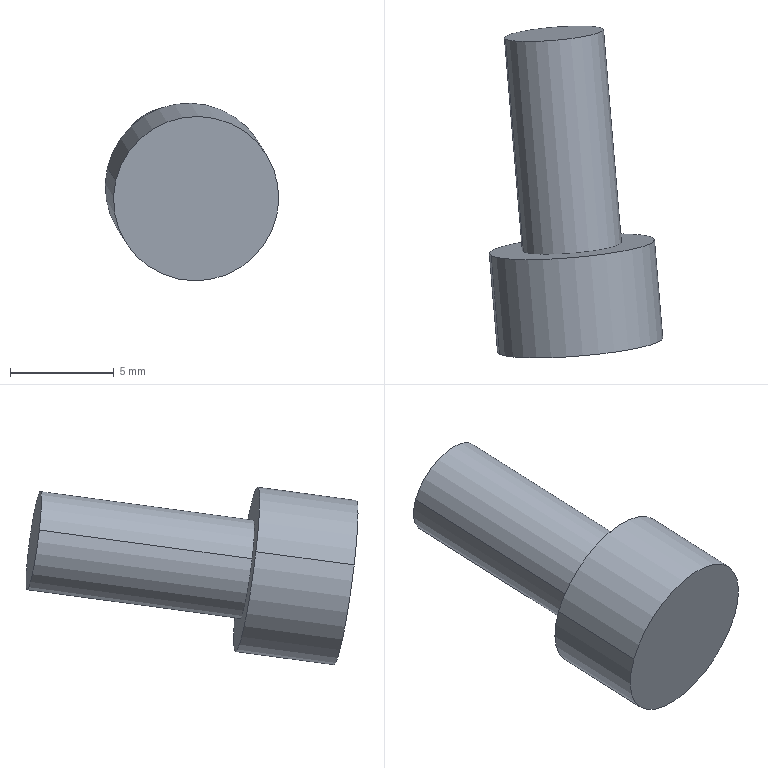Part | SolidWorks | features SplitBody 1 | 1 solid | 7 faces | box 8.371 x 16.016 x 8.568 mm | volume 429.468 mm3 | cylinder 4 | plane 3 | commonest cylinder face diameters 4.8 x2 8 x2
STEP:
#1=CARTESIAN_POINT('',(518.089,343.49,-353.855));
#2=VERTEX_POINT('',#1);
#3=CARTESIAN_POINT('',(522.748,344.02,-354.879));
#4=VERTEX_POINT('',#3);
#5=CARTESIAN_POINT('',(520.418,343.755,-354.367));
#6=DIRECTION('',(0.08315,-0.9876,-0.1332));
#7=DIRECTION('',(-0.9707,-0.1105,0.2133));
#8=AXIS2_PLACEMENT_3D('',#5,#6,#7);
#9=CIRCLE('',#8,2.4);
#10=EDGE_CURVE('',#2,#4,#9,.T.);
#11=ORIENTED_EDGE('',*,*,#10,.T.);
#12=CARTESIAN_POINT('',(523.613,333.749,-356.264));
#13=VERTEX_POINT('',#12);
#14=CARTESIAN_POINT('',(522.748,344.02,-354.879));
#15=DIRECTION('',(0.08315,-0.9876,-0.1332));
#16=VECTOR('',#15,1000.);
#17=LINE('',#14,#16);
#18=EDGE_CURVE('',#4,#13,#17,.T.);
#19=ORIENTED_EDGE('',*,*,#18,.T.);
#20=CARTESIAN_POINT('',(518.953,333.219,-355.24));
#21=VERTEX_POINT('',#20);
#22=CARTESIAN_POINT('',(521.283,333.484,-355.752));
#23=DIRECTION('',(0.08315,-0.9876,-0.1332));
#24=DIRECTION('',(-0.9707,-0.1105,0.2133));
#25=AXIS2_PLACEMENT_3D('',#22,#23,#24);
#26=CIRCLE('',#25,2.4);
#27=EDGE_CURVE('',#21,#13,#26,.T.);
#28=ORIENTED_EDGE('',*,*,#27,.F.);
#29=CARTESIAN_POINT('',(518.089,343.49,-353.855));
#30=DIRECTION('',(0.08315,-0.9876,-0.1332));
#31=VECTOR('',#30,1000.);
#32=LINE('',#29,#31);
#33=EDGE_CURVE('',#2,#21,#32,.T.);
#34=ORIENTED_EDGE('',*,*,#33,.F.);
#35=EDGE_LOOP('',(#11,#19,#28,#34));
#36=FACE_OUTER_BOUND('',#35,.T.);
#37=CARTESIAN_POINT('',(520.418,343.755,-354.367));
#38=DIRECTION('',(0.08315,-0.9876,-0.1332));
#39=DIRECTION('',(-0.9707,-0.1105,0.2133));
#40=AXIS2_PLACEMENT_3D('',#37,#38,#39);
#41=CYLINDRICAL_SURFACE('',#40,2.4);
#42=ADVANCED_FACE('',(#36),#41,.T.);
#43=CARTESIAN_POINT('',(517.799,328.302,-355.538));
#44=VERTEX_POINT('',#43);
#45=CARTESIAN_POINT('',(525.565,329.186,-357.245));
#46=VERTEX_POINT('',#45);
#47=CARTESIAN_POINT('',(521.682,328.744,-356.392));
#48=DIRECTION('',(0.08315,-0.9876,-0.1332));
#49=DIRECTION('',(-0.9707,-0.1105,0.2133));
#50=AXIS2_PLACEMENT_3D('',#47,#48,#49);
#51=CIRCLE('',#50,4.);
#52=EDGE_CURVE('',#44,#46,#51,.T.);
#53=ORIENTED_EDGE('',*,*,#52,.F.);
#54=CARTESIAN_POINT('',(517.4,333.042,-354.899));
#55=VERTEX_POINT('',#54);
#56=CARTESIAN_POINT('',(517.799,328.302,-355.538));
#57=DIRECTION('',(-0.08315,0.9876,0.1332));
#58=VECTOR('',#57,1000.);
#59=LINE('',#56,#58);
#60=EDGE_CURVE('',#44,#55,#59,.T.);
#61=ORIENTED_EDGE('',*,*,#60,.T.);
#62=CARTESIAN_POINT('',(525.166,333.926,-356.605));
#63=VERTEX_POINT('',#62);
#64=CARTESIAN_POINT('',(521.283,333.484,-355.752));
#65=DIRECTION('',(0.08315,-0.9876,-0.1332));
#66=DIRECTION('',(-0.9707,-0.1105,0.2133));
#67=AXIS2_PLACEMENT_3D('',#64,#65,#66);
#68=CIRCLE('',#67,4.);
#69=EDGE_CURVE('',#55,#63,#68,.T.);
#70=ORIENTED_EDGE('',*,*,#69,.T.);
#71=CARTESIAN_POINT('',(525.565,329.186,-357.245));
#72=DIRECTION('',(-0.08315,0.9876,0.1332));
#73=VECTOR('',#72,1000.);
#74=LINE('',#71,#73);
#75=EDGE_CURVE('',#46,#63,#74,.T.);
#76=ORIENTED_EDGE('',*,*,#75,.F.);
#77=EDGE_LOOP('',(#53,#61,#70,#76));
#78=FACE_OUTER_BOUND('',#77,.T.);
#79=CARTESIAN_POINT('',(521.682,328.744,-356.392));
#80=DIRECTION('',(-0.08315,0.9876,0.1332));
#81=DIRECTION('',(0.9707,0.1105,-0.2133));
#82=AXIS2_PLACEMENT_3D('',#79,#80,#81);
#83=CYLINDRICAL_SURFACE('',#82,4.);
#84=ADVANCED_FACE('',(#78),#83,.T.);
#85=ORIENTED_EDGE('',*,*,#60,.F.);
#86=CARTESIAN_POINT('',(521.682,328.744,-356.392));
#87=DIRECTION('',(0.08315,-0.9876,-0.1332));
#88=DIRECTION('',(-0.9707,-0.1105,0.2133));
#89=AXIS2_PLACEMENT_3D('',#86,#87,#88);
#90=CIRCLE('',#89,4.);
#91=EDGE_CURVE('',#46,#44,#90,.T.);
#92=ORIENTED_EDGE('',*,*,#91,.F.);
#93=ORIENTED_EDGE('',*,*,#75,.T.);
#94=CARTESIAN_POINT('',(521.283,333.484,-355.752));
#95=DIRECTION('',(0.08315,-0.9876,-0.1332));
#96=DIRECTION('',(-0.9707,-0.1105,0.2133));
#97=AXIS2_PLACEMENT_3D('',#94,#95,#96);
#98=CIRCLE('',#97,4.);
#99=EDGE_CURVE('',#63,#55,#98,.T.);
#100=ORIENTED_EDGE('',*,*,#99,.T.);
#101=EDGE_LOOP('',(#85,#92,#93,#100));
#102=FACE_OUTER_BOUND('',#101,.T.);
#103=CARTESIAN_POINT('',(521.682,328.744,-356.392));
#104=DIRECTION('',(-0.08315,0.9876,0.1332));
#105=DIRECTION('',(0.9707,0.1105,-0.2133));
#106=AXIS2_PLACEMENT_3D('',#103,#104,#105);
#107=CYLINDRICAL_SURFACE('',#106,4.);
#108=ADVANCED_FACE('',(#102),#107,.T.);
#109=ORIENTED_EDGE('',*,*,#91,.T.);
#110=ORIENTED_EDGE('',*,*,#52,.T.);
#111=EDGE_LOOP('',(#109,#110));
#112=FACE_OUTER_BOUND('',#111,.T.);
#113=CARTESIAN_POINT('',(521.682,328.744,-356.392));
#114=DIRECTION('',(0.08315,-0.9876,-0.1332));
#115=DIRECTION('',(-0.9707,-0.1105,0.2133));
#116=AXIS2_PLACEMENT_3D('',#113,#114,#115);
#117=PLANE('',#116);
#118=ADVANCED_FACE('',(#112),#117,.T.);
#119=ORIENTED_EDGE('',*,*,#27,.T.);
#120=CARTESIAN_POINT('',(521.283,333.484,-355.752));
#121=DIRECTION('',(0.08315,-0.9876,-0.1332));
#122=DIRECTION('',(-0.9707,-0.1105,0.2133));
#123=AXIS2_PLACEMENT_3D('',#120,#121,#122);
#124=CIRCLE('',#123,2.4);
#125=EDGE_CURVE('',#13,#21,#124,.T.);
#126=ORIENTED_EDGE('',*,*,#125,.T.);
#127=EDGE_LOOP('',(#119,#126));
#128=FACE_BOUND('',#127,.T.);
#129=ORIENTED_EDGE('',*,*,#99,.F.);
#130=ORIENTED_EDGE('',*,*,#69,.F.);
#131=EDGE_LOOP('',(#129,#130));
#132=FACE_OUTER_BOUND('',#131,.T.);
#133=CARTESIAN_POINT('',(521.283,333.484,-355.752));
#134=DIRECTION('',(0.08315,-0.9876,-0.1332));
#135=DIRECTION('',(-0.9707,-0.1105,0.2133));
#136=AXIS2_PLACEMENT_3D('',#133,#134,#135);
#137=PLANE('',#136);
#138=ADVANCED_FACE('',(#128,#132),#137,.F.);
#139=ORIENTED_EDGE('',*,*,#18,.F.);
#140=CARTESIAN_POINT('',(520.418,343.755,-354.367));
#141=DIRECTION('',(0.08315,-0.9876,-0.1332));
#142=DIRECTION('',(-0.9707,-0.1105,0.2133));
#143=AXIS2_PLACEMENT_3D('',#140,#141,#142);
#144=CIRCLE('',#143,2.4);
#145=EDGE_CURVE('',#4,#2,#144,.T.);
#146=ORIENTED_EDGE('',*,*,#145,.T.);
#147=ORIENTED_EDGE('',*,*,#33,.T.);
#148=ORIENTED_EDGE('',*,*,#125,.F.);
#149=EDGE_LOOP('',(#139,#146,#147,#148));
#150=FACE_OUTER_BOUND('',#149,.T.);
#151=CARTESIAN_POINT('',(520.418,343.755,-354.367));
#152=DIRECTION('',(0.08315,-0.9876,-0.1332));
#153=DIRECTION('',(-0.9707,-0.1105,0.2133));
#154=AXIS2_PLACEMENT_3D('',#151,#152,#153);
#155=CYLINDRICAL_SURFACE('',#154,2.4);
#156=ADVANCED_FACE('',(#150),#155,.T.);
#157=ORIENTED_EDGE('',*,*,#10,.F.);
#158=ORIENTED_EDGE('',*,*,#145,.F.);
#159=EDGE_LOOP('',(#157,#158));
#160=FACE_OUTER_BOUND('',#159,.T.);
#161=CARTESIAN_POINT('',(520.418,343.755,-354.367));
#162=DIRECTION('',(0.08315,-0.9876,-0.1332));
#163=DIRECTION('',(-0.9707,-0.1105,0.2133));
#164=AXIS2_PLACEMENT_3D('',#161,#162,#163);
#165=PLANE('',#164);
#166=ADVANCED_FACE('',(#160),#165,.F.);
#167=CLOSED_SHELL('',(#42,#84,#108,#118,#138,#156,#166));
#168=MANIFOLD_SOLID_BREP('',#167);
#169=CARTESIAN_POINT('',(0.,0.,0.));
#170=DIRECTION('',(0.,0.,1.));
#171=DIRECTION('',(1.,0.,0.));
#172=AXIS2_PLACEMENT_3D('',#169,#170,#171);
#173=(LENGTH_UNIT()NAMED_UNIT(*)SI_UNIT(.MILLI.,.METRE.));
#174=UNCERTAINTY_MEASURE_WITH_UNIT(LENGTH_MEASURE(0.00001),#173,'','');
#175=(NAMED_UNIT(*)PLANE_ANGLE_UNIT()SI_UNIT($,.RADIAN.));
#176=(NAMED_UNIT(*)SI_UNIT($,.STERADIAN.)SOLID_ANGLE_UNIT());
#177=(GEOMETRIC_REPRESENTATION_CONTEXT(3)GLOBAL_UNCERTAINTY_ASSIGNED_CONTEXT((#174))GLOBAL_UNIT_ASSIGNED_CONTEXT((#173,#175,#176))REPRESENTATION_CONTEXT('',''));
#178=ADVANCED_BREP_SHAPE_REPRESENTATION('',(#168,#172),#177);